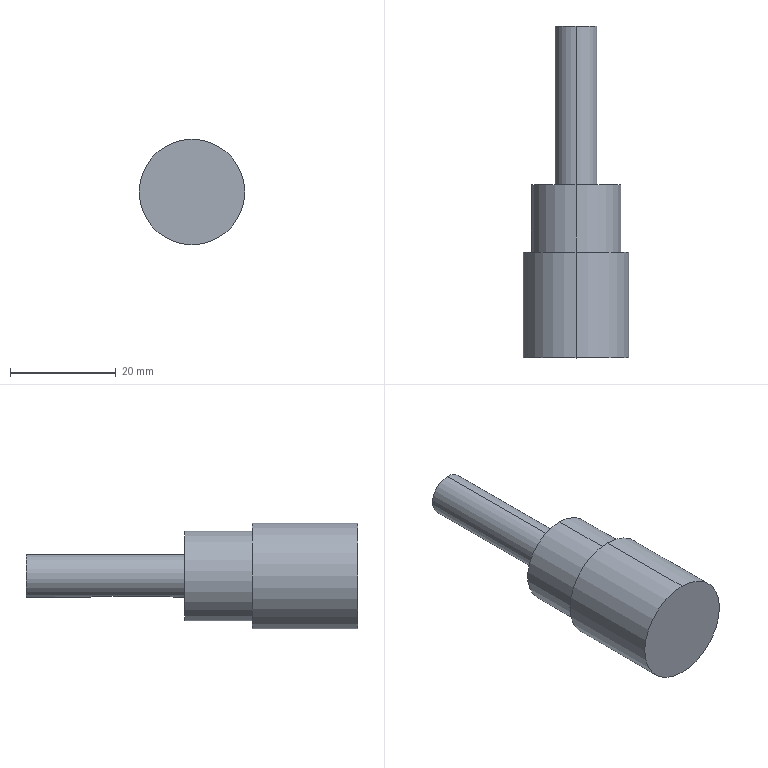Part | SolidWorks | features ICE 3, Extrusion 1 | 1 solid | 15 faces | box 20 x 62.8 x 20 mm | volume 10660 mm3 | cylinder 8 | plane 7 | commonest cylinder face diameters 2 x2 8 x2 17 x2 20 x2
STEP:
#1=CARTESIAN_POINT('',(0.,62.8,4.));
#2=VERTEX_POINT('',#1);
#3=CARTESIAN_POINT('',(0.,62.8,-4.));
#4=VERTEX_POINT('',#3);
#5=CARTESIAN_POINT('',(0.,62.8,0.));
#6=DIRECTION('',(0.,1.,0.));
#7=DIRECTION('',(0.,0.,1.));
#8=AXIS2_PLACEMENT_3D('',#5,#6,#7);
#9=CIRCLE('',#8,4.);
#10=EDGE_CURVE('',#2,#4,#9,.T.);
#11=ORIENTED_EDGE('',*,*,#10,.F.);
#12=CARTESIAN_POINT('',(0.,32.8,4.));
#13=VERTEX_POINT('',#12);
#14=CARTESIAN_POINT('',(0.,62.8,4.));
#15=DIRECTION('',(0.,-1.,0.));
#16=VECTOR('',#15,1000.);
#17=LINE('',#14,#16);
#18=EDGE_CURVE('',#2,#13,#17,.T.);
#19=ORIENTED_EDGE('',*,*,#18,.T.);
#20=CARTESIAN_POINT('',(0.,32.8,-4.));
#21=VERTEX_POINT('',#20);
#22=CARTESIAN_POINT('',(0.,32.8,0.));
#23=DIRECTION('',(0.,1.,0.));
#24=DIRECTION('',(0.,0.,1.));
#25=AXIS2_PLACEMENT_3D('',#22,#23,#24);
#26=CIRCLE('',#25,4.);
#27=EDGE_CURVE('',#13,#21,#26,.T.);
#28=ORIENTED_EDGE('',*,*,#27,.T.);
#29=CARTESIAN_POINT('',(0.,34.8,-4.));
#30=VERTEX_POINT('',#29);
#31=CARTESIAN_POINT('',(0.,62.8,-4.));
#32=DIRECTION('',(0.,-1.,0.));
#33=VECTOR('',#32,1000.);
#34=LINE('',#31,#33);
#35=EDGE_CURVE('',#30,#21,#34,.T.);
#36=ORIENTED_EDGE('',*,*,#35,.F.);
#37=CARTESIAN_POINT('',(1.,35.8,-3.873));
#38=VERTEX_POINT('',#37);
#39=CARTESIAN_POINT('',(0.,34.8,-4.));
#40=CARTESIAN_POINT('',(0.1309,34.8,-4.));
#41=CARTESIAN_POINT('',(0.2621,34.826,-3.993));
#42=CARTESIAN_POINT('',(0.5047,34.927,-3.97));
#43=CARTESIAN_POINT('',(0.6146,35.,-3.954));
#44=CARTESIAN_POINT('',(0.7997,35.185,-3.92));
#45=CARTESIAN_POINT('',(0.8733,35.296,-3.904));
#46=CARTESIAN_POINT('',(0.9735,35.537,-3.88));
#47=CARTESIAN_POINT('',(1.,35.667,-3.873));
#48=CARTESIAN_POINT('',(1.,35.8,-3.873));
#49=B_SPLINE_CURVE_WITH_KNOTS('',3,(#39,#40,#41,#42,#43,#44,#45,#46,#47,#48),.UNSPECIFIED.,.F.,.F.,(4,2,2,2,4),(0.00157,0.001962,0.002354,0.002746,0.003138),.UNSPECIFIED.);
#50=EDGE_CURVE('',#30,#38,#49,.T.);
#51=ORIENTED_EDGE('',*,*,#50,.T.);
#52=CARTESIAN_POINT('',(1.,49.8,-3.873));
#53=VERTEX_POINT('',#52);
#54=CARTESIAN_POINT('',(1.,62.8,-3.873));
#55=DIRECTION('',(0.,1.,0.));
#56=VECTOR('',#55,1000.);
#57=LINE('',#54,#56);
#58=EDGE_CURVE('',#38,#53,#57,.T.);
#59=ORIENTED_EDGE('',*,*,#58,.T.);
#60=CARTESIAN_POINT('',(0.,50.8,-4.));
#61=VERTEX_POINT('',#60);
#62=CARTESIAN_POINT('',(1.,49.8,-3.873));
#63=CARTESIAN_POINT('',(1.,49.933,-3.873));
#64=CARTESIAN_POINT('',(0.9737,50.063,-3.88));
#65=CARTESIAN_POINT('',(0.873,50.305,-3.904));
#66=CARTESIAN_POINT('',(0.7987,50.416,-3.921));
#67=CARTESIAN_POINT('',(0.6149,50.599,-3.954));
#68=CARTESIAN_POINT('',(0.5037,50.674,-3.97));
#69=CARTESIAN_POINT('',(0.2631,50.774,-3.993));
#70=CARTESIAN_POINT('',(0.1311,50.8,-4.));
#71=CARTESIAN_POINT('',(0.,50.8,-4.));
#72=B_SPLINE_CURVE_WITH_KNOTS('',3,(#62,#63,#64,#65,#66,#67,#68,#69,#70,#71),.UNSPECIFIED.,.F.,.F.,(4,2,2,2,4),(0.,0.0003925,0.0007849,0.001177,0.00157),.UNSPECIFIED.);
#73=EDGE_CURVE('',#53,#61,#72,.T.);
#74=ORIENTED_EDGE('',*,*,#73,.T.);
#75=CARTESIAN_POINT('',(0.,62.8,-4.));
#76=DIRECTION('',(0.,-1.,0.));
#77=VECTOR('',#76,1000.);
#78=LINE('',#75,#77);
#79=EDGE_CURVE('',#4,#61,#78,.T.);
#80=ORIENTED_EDGE('',*,*,#79,.F.);
#81=EDGE_LOOP('',(#11,#19,#28,#36,#51,#59,#74,#80));
#82=FACE_OUTER_BOUND('',#81,.T.);
#83=CARTESIAN_POINT('',(0.,62.8,0.));
#84=DIRECTION('',(0.,-1.,0.));
#85=DIRECTION('',(0.,0.,-1.));
#86=AXIS2_PLACEMENT_3D('',#83,#84,#85);
#87=CYLINDRICAL_SURFACE('',#86,4.);
#88=ADVANCED_FACE('',(#82),#87,.T.);
#89=CARTESIAN_POINT('',(0.,32.8,8.5));
#90=VERTEX_POINT('',#89);
#91=CARTESIAN_POINT('',(0.,32.8,-8.5));
#92=VERTEX_POINT('',#91);
#93=CARTESIAN_POINT('',(0.,32.8,0.));
#94=DIRECTION('',(0.,1.,0.));
#95=DIRECTION('',(0.,0.,1.));
#96=AXIS2_PLACEMENT_3D('',#93,#94,#95);
#97=CIRCLE('',#96,8.5);
#98=EDGE_CURVE('',#90,#92,#97,.T.);
#99=ORIENTED_EDGE('',*,*,#98,.F.);
#100=CARTESIAN_POINT('',(0.,20.,8.5));
#101=VERTEX_POINT('',#100);
#102=CARTESIAN_POINT('',(0.,32.8,8.5));
#103=DIRECTION('',(0.,-1.,0.));
#104=VECTOR('',#103,1000.);
#105=LINE('',#102,#104);
#106=EDGE_CURVE('',#90,#101,#105,.T.);
#107=ORIENTED_EDGE('',*,*,#106,.T.);
#108=CARTESIAN_POINT('',(0.,20.,-8.5));
#109=VERTEX_POINT('',#108);
#110=CARTESIAN_POINT('',(0.,20.,0.));
#111=DIRECTION('',(0.,1.,0.));
#112=DIRECTION('',(0.,0.,1.));
#113=AXIS2_PLACEMENT_3D('',#110,#111,#112);
#114=CIRCLE('',#113,8.5);
#115=EDGE_CURVE('',#101,#109,#114,.T.);
#116=ORIENTED_EDGE('',*,*,#115,.T.);
#117=CARTESIAN_POINT('',(0.,32.8,-8.5));
#118=DIRECTION('',(0.,-1.,0.));
#119=VECTOR('',#118,1000.);
#120=LINE('',#117,#119);
#121=EDGE_CURVE('',#92,#109,#120,.T.);
#122=ORIENTED_EDGE('',*,*,#121,.F.);
#123=EDGE_LOOP('',(#99,#107,#116,#122));
#124=FACE_OUTER_BOUND('',#123,.T.);
#125=CARTESIAN_POINT('',(0.,32.8,0.));
#126=DIRECTION('',(0.,-1.,0.));
#127=DIRECTION('',(0.,0.,-1.));
#128=AXIS2_PLACEMENT_3D('',#125,#126,#127);
#129=CYLINDRICAL_SURFACE('',#128,8.5);
#130=ADVANCED_FACE('',(#124),#129,.T.);
#131=CARTESIAN_POINT('',(0.,20.,10.));
#132=VERTEX_POINT('',#131);
#133=CARTESIAN_POINT('',(0.,20.,-10.));
#134=VERTEX_POINT('',#133);
#135=CARTESIAN_POINT('',(0.,20.,0.));
#136=DIRECTION('',(0.,1.,0.));
#137=DIRECTION('',(0.,0.,1.));
#138=AXIS2_PLACEMENT_3D('',#135,#136,#137);
#139=CIRCLE('',#138,10.);
#140=EDGE_CURVE('',#132,#134,#139,.T.);
#141=ORIENTED_EDGE('',*,*,#140,.F.);
#142=CARTESIAN_POINT('',(0.,0.,10.));
#143=VERTEX_POINT('',#142);
#144=CARTESIAN_POINT('',(0.,20.,10.));
#145=DIRECTION('',(0.,-1.,0.));
#146=VECTOR('',#145,1000.);
#147=LINE('',#144,#146);
#148=EDGE_CURVE('',#132,#143,#147,.T.);
#149=ORIENTED_EDGE('',*,*,#148,.T.);
#150=CARTESIAN_POINT('',(0.,0.,-10.));
#151=VERTEX_POINT('',#150);
#152=CARTESIAN_POINT('',(0.,0.,0.));
#153=DIRECTION('',(0.,1.,0.));
#154=DIRECTION('',(0.,0.,1.));
#155=AXIS2_PLACEMENT_3D('',#152,#153,#154);
#156=CIRCLE('',#155,10.);
#157=EDGE_CURVE('',#143,#151,#156,.T.);
#158=ORIENTED_EDGE('',*,*,#157,.T.);
#159=CARTESIAN_POINT('',(0.,20.,-10.));
#160=DIRECTION('',(0.,-1.,0.));
#161=VECTOR('',#160,1000.);
#162=LINE('',#159,#161);
#163=EDGE_CURVE('',#134,#151,#162,.T.);
#164=ORIENTED_EDGE('',*,*,#163,.F.);
#165=EDGE_LOOP('',(#141,#149,#158,#164));
#166=FACE_OUTER_BOUND('',#165,.T.);
#167=CARTESIAN_POINT('',(0.,20.,0.));
#168=DIRECTION('',(0.,-1.,0.));
#169=DIRECTION('',(0.,0.,-1.));
#170=AXIS2_PLACEMENT_3D('',#167,#168,#169);
#171=CYLINDRICAL_SURFACE('',#170,10.);
#172=ADVANCED_FACE('',(#166),#171,.T.);
#173=ORIENTED_EDGE('',*,*,#148,.F.);
#174=CARTESIAN_POINT('',(0.,20.,0.));
#175=DIRECTION('',(0.,1.,0.));
#176=DIRECTION('',(0.,0.,1.));
#177=AXIS2_PLACEMENT_3D('',#174,#175,#176);
#178=CIRCLE('',#177,10.);
#179=EDGE_CURVE('',#134,#132,#178,.T.);
#180=ORIENTED_EDGE('',*,*,#179,.F.);
#181=ORIENTED_EDGE('',*,*,#163,.T.);
#182=CARTESIAN_POINT('',(0.,0.,0.));
#183=DIRECTION('',(0.,1.,0.));
#184=DIRECTION('',(0.,0.,1.));
#185=AXIS2_PLACEMENT_3D('',#182,#183,#184);
#186=CIRCLE('',#185,10.);
#187=EDGE_CURVE('',#151,#143,#186,.T.);
#188=ORIENTED_EDGE('',*,*,#187,.T.);
#189=EDGE_LOOP('',(#173,#180,#181,#188));
#190=FACE_OUTER_BOUND('',#189,.T.);
#191=CARTESIAN_POINT('',(0.,20.,0.));
#192=DIRECTION('',(0.,-1.,0.));
#193=DIRECTION('',(0.,0.,-1.));
#194=AXIS2_PLACEMENT_3D('',#191,#192,#193);
#195=CYLINDRICAL_SURFACE('',#194,10.);
#196=ADVANCED_FACE('',(#190),#195,.T.);
#197=CARTESIAN_POINT('',(0.,20.,0.));
#198=DIRECTION('',(0.,1.,0.));
#199=DIRECTION('',(0.,0.,1.));
#200=AXIS2_PLACEMENT_3D('',#197,#198,#199);
#201=CIRCLE('',#200,8.5);
#202=EDGE_CURVE('',#109,#101,#201,.T.);
#203=ORIENTED_EDGE('',*,*,#202,.F.);
#204=ORIENTED_EDGE('',*,*,#115,.F.);
#205=EDGE_LOOP('',(#203,#204));
#206=FACE_BOUND('',#205,.T.);
#207=ORIENTED_EDGE('',*,*,#179,.T.);
#208=ORIENTED_EDGE('',*,*,#140,.T.);
#209=EDGE_LOOP('',(#207,#208));
#210=FACE_OUTER_BOUND('',#209,.T.);
#211=CARTESIAN_POINT('',(0.,20.,0.));
#212=DIRECTION('',(0.,1.,0.));
#213=DIRECTION('',(0.,0.,1.));
#214=AXIS2_PLACEMENT_3D('',#211,#212,#213);
#215=PLANE('',#214);
#216=ADVANCED_FACE('',(#206,#210),#215,.T.);
#217=ORIENTED_EDGE('',*,*,#187,.F.);
#218=ORIENTED_EDGE('',*,*,#157,.F.);
#219=EDGE_LOOP('',(#217,#218));
#220=FACE_OUTER_BOUND('',#219,.T.);
#221=CARTESIAN_POINT('',(0.,0.,0.));
#222=DIRECTION('',(0.,1.,0.));
#223=DIRECTION('',(0.,0.,1.));
#224=AXIS2_PLACEMENT_3D('',#221,#222,#223);
#225=PLANE('',#224);
#226=ADVANCED_FACE('',(#220),#225,.F.);
#227=ORIENTED_EDGE('',*,*,#106,.F.);
#228=CARTESIAN_POINT('',(0.,32.8,0.));
#229=DIRECTION('',(0.,1.,0.));
#230=DIRECTION('',(0.,0.,1.));
#231=AXIS2_PLACEMENT_3D('',#228,#229,#230);
#232=CIRCLE('',#231,8.5);
#233=EDGE_CURVE('',#92,#90,#232,.T.);
#234=ORIENTED_EDGE('',*,*,#233,.F.);
#235=ORIENTED_EDGE('',*,*,#121,.T.);
#236=ORIENTED_EDGE('',*,*,#202,.T.);
#237=EDGE_LOOP('',(#227,#234,#235,#236));
#238=FACE_OUTER_BOUND('',#237,.T.);
#239=CARTESIAN_POINT('',(0.,32.8,0.));
#240=DIRECTION('',(0.,-1.,0.));
#241=DIRECTION('',(0.,0.,-1.));
#242=AXIS2_PLACEMENT_3D('',#239,#240,#241);
#243=CYLINDRICAL_SURFACE('',#242,8.5);
#244=ADVANCED_FACE('',(#238),#243,.T.);
#245=CARTESIAN_POINT('',(0.,32.8,0.));
#246=DIRECTION('',(0.,1.,0.));
#247=DIRECTION('',(0.,0.,1.));
#248=AXIS2_PLACEMENT_3D('',#245,#246,#247);
#249=CIRCLE('',#248,4.);
#250=EDGE_CURVE('',#21,#13,#249,.T.);
#251=ORIENTED_EDGE('',*,*,#250,.F.);
#252=ORIENTED_EDGE('',*,*,#27,.F.);
#253=EDGE_LOOP('',(#251,#252));
#254=FACE_BOUND('',#253,.T.);
#255=ORIENTED_EDGE('',*,*,#233,.T.);
#256=ORIENTED_EDGE('',*,*,#98,.T.);
#257=EDGE_LOOP('',(#255,#256));
#258=FACE_OUTER_BOUND('',#257,.T.);
#259=CARTESIAN_POINT('',(0.,32.8,0.));
#260=DIRECTION('',(0.,1.,0.));
#261=DIRECTION('',(0.,0.,1.));
#262=AXIS2_PLACEMENT_3D('',#259,#260,#261);
#263=PLANE('',#262);
#264=ADVANCED_FACE('',(#254,#258),#263,.T.);
#265=ORIENTED_EDGE('',*,*,#18,.F.);
#266=CARTESIAN_POINT('',(0.,62.8,0.));
#267=DIRECTION('',(0.,1.,0.));
#268=DIRECTION('',(0.,0.,1.));
#269=AXIS2_PLACEMENT_3D('',#266,#267,#268);
#270=CIRCLE('',#269,4.);
#271=EDGE_CURVE('',#4,#2,#270,.T.);
#272=ORIENTED_EDGE('',*,*,#271,.F.);
#273=ORIENTED_EDGE('',*,*,#79,.T.);
#274=CARTESIAN_POINT('',(-1.,49.8,-3.873));
#275=VERTEX_POINT('',#274);
#276=CARTESIAN_POINT('',(0.,50.8,-4.));
#277=CARTESIAN_POINT('',(-0.1309,50.8,-4.));
#278=CARTESIAN_POINT('',(-0.2621,50.774,-3.993));
#279=CARTESIAN_POINT('',(-0.5047,50.673,-3.97));
#280=CARTESIAN_POINT('',(-0.6146,50.6,-3.954));
#281=CARTESIAN_POINT('',(-0.7997,50.415,-3.92));
#282=CARTESIAN_POINT('',(-0.8733,50.304,-3.904));
#283=CARTESIAN_POINT('',(-0.9735,50.063,-3.88));
#284=CARTESIAN_POINT('',(-1.,49.933,-3.873));
#285=CARTESIAN_POINT('',(-1.,49.8,-3.873));
#286=B_SPLINE_CURVE_WITH_KNOTS('',3,(#276,#277,#278,#279,#280,#281,#282,#283,#284,#285),.UNSPECIFIED.,.F.,.F.,(4,2,2,2,4),(0.00157,0.001962,0.002354,0.002746,0.003138),.UNSPECIFIED.);
#287=EDGE_CURVE('',#61,#275,#286,.T.);
#288=ORIENTED_EDGE('',*,*,#287,.T.);
#289=CARTESIAN_POINT('',(-1.,35.8,-3.873));
#290=VERTEX_POINT('',#289);
#291=CARTESIAN_POINT('',(-1.,62.8,-3.873));
#292=DIRECTION('',(0.,-1.,0.));
#293=VECTOR('',#292,1000.);
#294=LINE('',#291,#293);
#295=EDGE_CURVE('',#275,#290,#294,.T.);
#296=ORIENTED_EDGE('',*,*,#295,.T.);
#297=CARTESIAN_POINT('',(-1.,35.8,-3.873));
#298=CARTESIAN_POINT('',(-1.,35.667,-3.873));
#299=CARTESIAN_POINT('',(-0.9737,35.537,-3.88));
#300=CARTESIAN_POINT('',(-0.873,35.295,-3.904));
#301=CARTESIAN_POINT('',(-0.7987,35.184,-3.921));
#302=CARTESIAN_POINT('',(-0.6149,35.001,-3.954));
#303=CARTESIAN_POINT('',(-0.5037,34.926,-3.97));
#304=CARTESIAN_POINT('',(-0.2631,34.826,-3.993));
#305=CARTESIAN_POINT('',(-0.1311,34.8,-4.));
#306=CARTESIAN_POINT('',(0.,34.8,-4.));
#307=B_SPLINE_CURVE_WITH_KNOTS('',3,(#297,#298,#299,#300,#301,#302,#303,#304,#305,#306),.UNSPECIFIED.,.F.,.F.,(4,2,2,2,4),(0.,0.0003925,0.0007849,0.001177,0.00157),.UNSPECIFIED.);
#308=EDGE_CURVE('',#290,#30,#307,.T.);
#309=ORIENTED_EDGE('',*,*,#308,.T.);
#310=ORIENTED_EDGE('',*,*,#35,.T.);
#311=ORIENTED_EDGE('',*,*,#250,.T.);
#312=EDGE_LOOP('',(#265,#272,#273,#288,#296,#309,#310,#311));
#313=FACE_OUTER_BOUND('',#312,.T.);
#314=CARTESIAN_POINT('',(0.,62.8,0.));
#315=DIRECTION('',(0.,-1.,0.));
#316=DIRECTION('',(0.,0.,-1.));
#317=AXIS2_PLACEMENT_3D('',#314,#315,#316);
#318=CYLINDRICAL_SURFACE('',#317,4.);
#319=ADVANCED_FACE('',(#313),#318,.T.);
#320=ORIENTED_EDGE('',*,*,#271,.T.);
#321=ORIENTED_EDGE('',*,*,#10,.T.);
#322=EDGE_LOOP('',(#320,#321));
#323=FACE_OUTER_BOUND('',#322,.T.);
#324=CARTESIAN_POINT('',(0.,62.8,0.));
#325=DIRECTION('',(0.,1.,0.));
#326=DIRECTION('',(0.,0.,1.));
#327=AXIS2_PLACEMENT_3D('',#324,#325,#326);
#328=PLANE('',#327);
#329=ADVANCED_FACE('',(#323),#328,.T.);
#330=CARTESIAN_POINT('',(1.,49.8,-2.8));
#331=VERTEX_POINT('',#330);
#332=CARTESIAN_POINT('',(1.,49.8,-2.8));
#333=DIRECTION('',(0.,0.,-1.));
#334=VECTOR('',#333,1000.);
#335=LINE('',#332,#334);
#336=EDGE_CURVE('',#331,#53,#335,.T.);
#337=ORIENTED_EDGE('',*,*,#336,.F.);
#338=CARTESIAN_POINT('',(-1.,49.8,-2.8));
#339=VERTEX_POINT('',#338);
#340=CARTESIAN_POINT('',(0.,49.8,-2.8));
#341=DIRECTION('',(0.,0.,-1.));
#342=DIRECTION('',(-1.,0.,0.));
#343=AXIS2_PLACEMENT_3D('',#340,#341,#342);
#344=CIRCLE('',#343,1.);
#345=EDGE_CURVE('',#339,#331,#344,.T.);
#346=ORIENTED_EDGE('',*,*,#345,.F.);
#347=CARTESIAN_POINT('',(-1.,49.8,-2.8));
#348=DIRECTION('',(0.,0.,-1.));
#349=VECTOR('',#348,1000.);
#350=LINE('',#347,#349);
#351=EDGE_CURVE('',#339,#275,#350,.T.);
#352=ORIENTED_EDGE('',*,*,#351,.T.);
#353=ORIENTED_EDGE('',*,*,#287,.F.);
#354=ORIENTED_EDGE('',*,*,#73,.F.);
#355=EDGE_LOOP('',(#337,#346,#352,#353,#354));
#356=FACE_OUTER_BOUND('',#355,.T.);
#357=CARTESIAN_POINT('',(0.,49.8,-2.8));
#358=DIRECTION('',(0.,0.,-1.));
#359=DIRECTION('',(-1.,0.,0.));
#360=AXIS2_PLACEMENT_3D('',#357,#358,#359);
#361=CYLINDRICAL_SURFACE('',#360,1.);
#362=ADVANCED_FACE('',(#356),#361,.F.);
#363=ORIENTED_EDGE('',*,*,#351,.F.);
#364=CARTESIAN_POINT('',(-1.,35.8,-2.8));
#365=VERTEX_POINT('',#364);
#366=CARTESIAN_POINT('',(-1.,49.8,-2.8));
#367=DIRECTION('',(0.,1.,0.));
#368=VECTOR('',#367,1000.);
#369=LINE('',#366,#368);
#370=EDGE_CURVE('',#365,#339,#369,.T.);
#371=ORIENTED_EDGE('',*,*,#370,.F.);
#372=CARTESIAN_POINT('',(-1.,35.8,-2.8));
#373=DIRECTION('',(0.,0.,-1.));
#374=VECTOR('',#373,1000.);
#375=LINE('',#372,#374);
#376=EDGE_CURVE('',#365,#290,#375,.T.);
#377=ORIENTED_EDGE('',*,*,#376,.T.);
#378=ORIENTED_EDGE('',*,*,#295,.F.);
#379=EDGE_LOOP('',(#363,#371,#377,#378));
#380=FACE_OUTER_BOUND('',#379,.T.);
#381=CARTESIAN_POINT('',(-1.,49.8,-2.8));
#382=DIRECTION('',(-1.,0.,0.));
#383=DIRECTION('',(0.,-1.,0.));
#384=AXIS2_PLACEMENT_3D('',#381,#382,#383);
#385=PLANE('',#384);
#386=ADVANCED_FACE('',(#380),#385,.F.);
#387=ORIENTED_EDGE('',*,*,#376,.F.);
#388=CARTESIAN_POINT('',(1.,35.8,-2.8));
#389=VERTEX_POINT('',#388);
#390=CARTESIAN_POINT('',(0.,35.8,-2.8));
#391=DIRECTION('',(0.,0.,-1.));
#392=DIRECTION('',(-1.,0.,0.));
#393=AXIS2_PLACEMENT_3D('',#390,#391,#392);
#394=CIRCLE('',#393,1.);
#395=EDGE_CURVE('',#389,#365,#394,.T.);
#396=ORIENTED_EDGE('',*,*,#395,.F.);
#397=CARTESIAN_POINT('',(1.,35.8,-2.8));
#398=DIRECTION('',(0.,0.,-1.));
#399=VECTOR('',#398,1000.);
#400=LINE('',#397,#399);
#401=EDGE_CURVE('',#389,#38,#400,.T.);
#402=ORIENTED_EDGE('',*,*,#401,.T.);
#403=ORIENTED_EDGE('',*,*,#50,.F.);
#404=ORIENTED_EDGE('',*,*,#308,.F.);
#405=EDGE_LOOP('',(#387,#396,#402,#403,#404));
#406=FACE_OUTER_BOUND('',#405,.T.);
#407=CARTESIAN_POINT('',(0.,35.8,-2.8));
#408=DIRECTION('',(0.,0.,-1.));
#409=DIRECTION('',(-1.,0.,0.));
#410=AXIS2_PLACEMENT_3D('',#407,#408,#409);
#411=CYLINDRICAL_SURFACE('',#410,1.);
#412=ADVANCED_FACE('',(#406),#411,.F.);
#413=ORIENTED_EDGE('',*,*,#401,.F.);
#414=CARTESIAN_POINT('',(1.,49.8,-2.8));
#415=DIRECTION('',(0.,-1.,0.));
#416=VECTOR('',#415,1000.);
#417=LINE('',#414,#416);
#418=EDGE_CURVE('',#331,#389,#417,.T.);
#419=ORIENTED_EDGE('',*,*,#418,.F.);
#420=ORIENTED_EDGE('',*,*,#336,.T.);
#421=ORIENTED_EDGE('',*,*,#58,.F.);
#422=EDGE_LOOP('',(#413,#419,#420,#421));
#423=FACE_OUTER_BOUND('',#422,.T.);
#424=CARTESIAN_POINT('',(1.,49.8,-2.8));
#425=DIRECTION('',(1.,0.,0.));
#426=DIRECTION('',(0.,1.,0.));
#427=AXIS2_PLACEMENT_3D('',#424,#425,#426);
#428=PLANE('',#427);
#429=ADVANCED_FACE('',(#423),#428,.F.);
#430=ORIENTED_EDGE('',*,*,#345,.T.);
#431=ORIENTED_EDGE('',*,*,#418,.T.);
#432=ORIENTED_EDGE('',*,*,#395,.T.);
#433=ORIENTED_EDGE('',*,*,#370,.T.);
#434=EDGE_LOOP('',(#430,#431,#432,#433));
#435=FACE_OUTER_BOUND('',#434,.T.);
#436=CARTESIAN_POINT('',(0.,49.8,-2.8));
#437=DIRECTION('',(0.,0.,-1.));
#438=DIRECTION('',(-1.,0.,0.));
#439=AXIS2_PLACEMENT_3D('',#436,#437,#438);
#440=PLANE('',#439);
#441=ADVANCED_FACE('',(#435),#440,.T.);
#442=CLOSED_SHELL('',(#88,#130,#172,#196,#216,#226,#244,#264,#319,#329,#362,#386,#412,#429,#441));
#443=MANIFOLD_SOLID_BREP('',#442);
#444=CARTESIAN_POINT('',(0.,0.,0.));
#445=DIRECTION('',(0.,0.,1.));
#446=DIRECTION('',(1.,0.,0.));
#447=AXIS2_PLACEMENT_3D('',#444,#445,#446);
#448=(LENGTH_UNIT()NAMED_UNIT(*)SI_UNIT(.MILLI.,.METRE.));
#449=UNCERTAINTY_MEASURE_WITH_UNIT(LENGTH_MEASURE(0.00001),#448,'','');
#450=(NAMED_UNIT(*)PLANE_ANGLE_UNIT()SI_UNIT($,.RADIAN.));
#451=(NAMED_UNIT(*)SI_UNIT($,.STERADIAN.)SOLID_ANGLE_UNIT());
#452=(GEOMETRIC_REPRESENTATION_CONTEXT(3)GLOBAL_UNCERTAINTY_ASSIGNED_CONTEXT((#449))GLOBAL_UNIT_ASSIGNED_CONTEXT((#448,#450,#451))REPRESENTATION_CONTEXT('',''));
#453=ADVANCED_BREP_SHAPE_REPRESENTATION('',(#443,#447),#452);